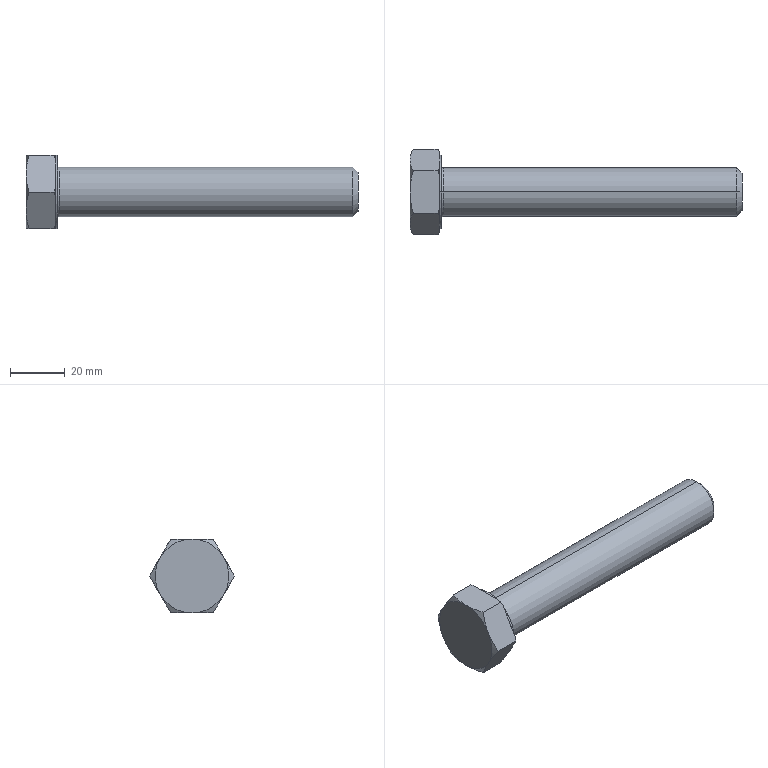Part | SolidWorks | features RevCut 4, Chamfer 1, Extrusion 1, Fillet 1, LPattern 1, Revolution 1 | 1 solid | 35 faces | box 121.5 x 31.177 x 27 mm | volume 35083 mm3 | plane 15 | cone 14 | cylinder 4 | torus 2 | commonest cylinder face diameters 18 x2 27 x2
STEP:
#1=CARTESIAN_POINT('',(12.1,0.,9.));
#2=VERTEX_POINT('',#1);
#3=CARTESIAN_POINT('',(12.1,0.,-9.));
#4=VERTEX_POINT('',#3);
#5=CARTESIAN_POINT('',(12.1,0.,0.));
#6=DIRECTION('',(1.,0.,0.));
#7=DIRECTION('',(0.,0.,-1.));
#8=AXIS2_PLACEMENT_3D('',#5,#6,#7);
#9=CIRCLE('',#8,9.);
#10=EDGE_CURVE('',#2,#4,#9,.T.);
#11=ORIENTED_EDGE('',*,*,#10,.F.);
#12=CARTESIAN_POINT('',(11.5,0.,9.6));
#13=VERTEX_POINT('',#12);
#14=CARTESIAN_POINT('',(12.1,0.,9.6));
#15=DIRECTION('',(0.,1.,0.));
#16=DIRECTION('',(0.,0.,1.));
#17=AXIS2_PLACEMENT_3D('',#14,#15,#16);
#18=CIRCLE('',#17,0.6);
#19=EDGE_CURVE('',#2,#13,#18,.T.);
#20=ORIENTED_EDGE('',*,*,#19,.T.);
#21=CARTESIAN_POINT('',(11.5,0.,-9.6));
#22=VERTEX_POINT('',#21);
#23=CARTESIAN_POINT('',(11.5,0.,0.));
#24=DIRECTION('',(-1.,0.,0.));
#25=DIRECTION('',(0.,0.,-1.));
#26=AXIS2_PLACEMENT_3D('',#23,#24,#25);
#27=CIRCLE('',#26,9.6);
#28=EDGE_CURVE('',#22,#13,#27,.T.);
#29=ORIENTED_EDGE('',*,*,#28,.F.);
#30=CARTESIAN_POINT('',(12.1,0.,-9.6));
#31=DIRECTION('',(0.,-1.,0.));
#32=DIRECTION('',(0.,0.,-1.));
#33=AXIS2_PLACEMENT_3D('',#30,#31,#32);
#34=CIRCLE('',#33,0.6);
#35=EDGE_CURVE('',#4,#22,#34,.T.);
#36=ORIENTED_EDGE('',*,*,#35,.F.);
#37=EDGE_LOOP('',(#11,#20,#29,#36));
#38=FACE_OUTER_BOUND('',#37,.T.);
#39=CARTESIAN_POINT('',(12.1,0.,0.));
#40=DIRECTION('',(1.,0.,0.));
#41=DIRECTION('',(0.,0.,-1.));
#42=AXIS2_PLACEMENT_3D('',#39,#40,#41);
#43=TOROIDAL_SURFACE('',#42,9.6,0.6);
#44=ADVANCED_FACE('',(#38),#43,.F.);
#45=CARTESIAN_POINT('',(121.5,0.,-7.));
#46=VERTEX_POINT('',#45);
#47=CARTESIAN_POINT('',(121.5,0.,7.));
#48=VERTEX_POINT('',#47);
#49=CARTESIAN_POINT('',(121.5,0.,0.));
#50=DIRECTION('',(1.,0.,0.));
#51=DIRECTION('',(0.,0.,1.));
#52=AXIS2_PLACEMENT_3D('',#49,#50,#51);
#53=CIRCLE('',#52,7.);
#54=EDGE_CURVE('',#46,#48,#53,.T.);
#55=ORIENTED_EDGE('',*,*,#54,.F.);
#56=CARTESIAN_POINT('',(119.5,0.,-9.));
#57=VERTEX_POINT('',#56);
#58=CARTESIAN_POINT('',(119.5,0.,-9.));
#59=DIRECTION('',(-0.7071,0.,-0.7071));
#60=VECTOR('',#59,1000.);
#61=LINE('',#58,#60);
#62=EDGE_CURVE('',#46,#57,#61,.T.);
#63=ORIENTED_EDGE('',*,*,#62,.T.);
#64=CARTESIAN_POINT('',(119.5,0.,9.));
#65=VERTEX_POINT('',#64);
#66=CARTESIAN_POINT('',(119.5,0.,0.));
#67=DIRECTION('',(-1.,0.,0.));
#68=DIRECTION('',(0.,0.,1.));
#69=AXIS2_PLACEMENT_3D('',#66,#67,#68);
#70=CIRCLE('',#69,9.);
#71=EDGE_CURVE('',#65,#57,#70,.T.);
#72=ORIENTED_EDGE('',*,*,#71,.F.);
#73=CARTESIAN_POINT('',(119.5,0.,9.));
#74=DIRECTION('',(-0.7071,0.,0.7071));
#75=VECTOR('',#74,1000.);
#76=LINE('',#73,#75);
#77=EDGE_CURVE('',#48,#65,#76,.T.);
#78=ORIENTED_EDGE('',*,*,#77,.F.);
#79=EDGE_LOOP('',(#55,#63,#72,#78));
#80=FACE_OUTER_BOUND('',#79,.T.);
#81=CARTESIAN_POINT('',(119.5,0.,0.));
#82=DIRECTION('',(-1.,0.,0.));
#83=DIRECTION('',(0.,0.,1.));
#84=AXIS2_PLACEMENT_3D('',#81,#82,#83);
#85=CONICAL_SURFACE('',#84,9.,0.7854);
#86=ADVANCED_FACE('',(#80),#85,.T.);
#87=ORIENTED_EDGE('',*,*,#71,.T.);
#88=CARTESIAN_POINT('',(0.,0.,-9.));
#89=DIRECTION('',(-1.,0.,0.));
#90=VECTOR('',#89,1000.);
#91=LINE('',#88,#90);
#92=EDGE_CURVE('',#57,#4,#91,.T.);
#93=ORIENTED_EDGE('',*,*,#92,.T.);
#94=CARTESIAN_POINT('',(12.1,0.,0.));
#95=DIRECTION('',(1.,0.,0.));
#96=DIRECTION('',(0.,0.,-1.));
#97=AXIS2_PLACEMENT_3D('',#94,#95,#96);
#98=CIRCLE('',#97,9.);
#99=EDGE_CURVE('',#4,#2,#98,.T.);
#100=ORIENTED_EDGE('',*,*,#99,.T.);
#101=CARTESIAN_POINT('',(0.,0.,9.));
#102=DIRECTION('',(-1.,0.,0.));
#103=VECTOR('',#102,1000.);
#104=LINE('',#101,#103);
#105=EDGE_CURVE('',#65,#2,#104,.T.);
#106=ORIENTED_EDGE('',*,*,#105,.F.);
#107=EDGE_LOOP('',(#87,#93,#100,#106));
#108=FACE_OUTER_BOUND('',#107,.T.);
#109=CARTESIAN_POINT('',(0.,0.,0.));
#110=DIRECTION('',(-1.,0.,0.));
#111=DIRECTION('',(0.,0.,1.));
#112=AXIS2_PLACEMENT_3D('',#109,#110,#111);
#113=CYLINDRICAL_SURFACE('',#112,9.);
#114=ADVANCED_FACE('',(#108),#113,.T.);
#115=CARTESIAN_POINT('',(11.5,0.,-13.5));
#116=VERTEX_POINT('',#115);
#117=CARTESIAN_POINT('',(11.5,0.,13.5));
#118=VERTEX_POINT('',#117);
#119=CARTESIAN_POINT('',(11.5,0.,0.));
#120=DIRECTION('',(1.,0.,0.));
#121=DIRECTION('',(0.,0.,-1.));
#122=AXIS2_PLACEMENT_3D('',#119,#120,#121);
#123=CIRCLE('',#122,13.5);
#124=EDGE_CURVE('',#116,#118,#123,.T.);
#125=ORIENTED_EDGE('',*,*,#124,.F.);
#126=CARTESIAN_POINT('',(10.7,0.,-13.5));
#127=VERTEX_POINT('',#126);
#128=CARTESIAN_POINT('',(0.,0.,-13.5));
#129=DIRECTION('',(-1.,0.,0.));
#130=VECTOR('',#129,1000.);
#131=LINE('',#128,#130);
#132=EDGE_CURVE('',#116,#127,#131,.T.);
#133=ORIENTED_EDGE('',*,*,#132,.T.);
#134=CARTESIAN_POINT('',(10.7,11.691,-6.75));
#135=VERTEX_POINT('',#134);
#136=CARTESIAN_POINT('',(10.7,0.,0.));
#137=DIRECTION('',(-1.,0.,0.));
#138=DIRECTION('',(0.,0.,1.));
#139=AXIS2_PLACEMENT_3D('',#136,#137,#138);
#140=CIRCLE('',#139,13.5);
#141=EDGE_CURVE('',#135,#127,#140,.T.);
#142=ORIENTED_EDGE('',*,*,#141,.F.);
#143=CARTESIAN_POINT('',(10.7,11.691,6.75));
#144=VERTEX_POINT('',#143);
#145=CARTESIAN_POINT('',(10.7,0.,0.));
#146=DIRECTION('',(-1.,0.,0.));
#147=DIRECTION('',(0.,0.,1.));
#148=AXIS2_PLACEMENT_3D('',#145,#146,#147);
#149=CIRCLE('',#148,13.5);
#150=EDGE_CURVE('',#144,#135,#149,.T.);
#151=ORIENTED_EDGE('',*,*,#150,.F.);
#152=CARTESIAN_POINT('',(10.7,0.,13.5));
#153=VERTEX_POINT('',#152);
#154=CARTESIAN_POINT('',(10.7,0.,0.));
#155=DIRECTION('',(-1.,0.,0.));
#156=DIRECTION('',(0.,0.,1.));
#157=AXIS2_PLACEMENT_3D('',#154,#155,#156);
#158=CIRCLE('',#157,13.5);
#159=EDGE_CURVE('',#153,#144,#158,.T.);
#160=ORIENTED_EDGE('',*,*,#159,.F.);
#161=CARTESIAN_POINT('',(0.,0.,13.5));
#162=DIRECTION('',(-1.,0.,0.));
#163=VECTOR('',#162,1000.);
#164=LINE('',#161,#163);
#165=EDGE_CURVE('',#118,#153,#164,.T.);
#166=ORIENTED_EDGE('',*,*,#165,.F.);
#167=EDGE_LOOP('',(#125,#133,#142,#151,#160,#166));
#168=FACE_OUTER_BOUND('',#167,.T.);
#169=CARTESIAN_POINT('',(0.,0.,0.));
#170=DIRECTION('',(-1.,0.,0.));
#171=DIRECTION('',(0.,0.,1.));
#172=AXIS2_PLACEMENT_3D('',#169,#170,#171);
#173=CYLINDRICAL_SURFACE('',#172,13.5);
#174=ADVANCED_FACE('',(#168),#173,.T.);
#175=CARTESIAN_POINT('',(10.7,8.556,-12.181));
#176=VERTEX_POINT('',#175);
#177=CARTESIAN_POINT('',(10.7,7.794,-13.5));
#178=DIRECTION('',(0.,0.5,0.866));
#179=VECTOR('',#178,1000.);
#180=LINE('',#177,#179);
#181=EDGE_CURVE('',#176,#135,#180,.T.);
#182=ORIENTED_EDGE('',*,*,#181,.F.);
#183=CARTESIAN_POINT('',(10.294,7.794,-13.5));
#184=VERTEX_POINT('',#183);
#185=CARTESIAN_POINT('',(10.294,7.794,-13.5));
#186=CARTESIAN_POINT('',(10.44,8.047,-13.062));
#187=CARTESIAN_POINT('',(10.576,8.301,-12.622));
#188=CARTESIAN_POINT('',(10.7,8.556,-12.181));
#189=B_SPLINE_CURVE_WITH_KNOTS('',3,(#185,#186,#187,#188),.UNSPECIFIED.,.F.,.F.,(4,4),(0.000000238,0.001565),.UNSPECIFIED.);
#190=EDGE_CURVE('',#184,#176,#189,.T.);
#191=ORIENTED_EDGE('',*,*,#190,.F.);
#192=CARTESIAN_POINT('',(1.206,7.794,-13.5));
#193=VERTEX_POINT('',#192);
#194=CARTESIAN_POINT('',(11.5,7.794,-13.5));
#195=DIRECTION('',(-1.,0.,0.));
#196=VECTOR('',#195,1000.);
#197=LINE('',#194,#196);
#198=EDGE_CURVE('',#184,#193,#197,.T.);
#199=ORIENTED_EDGE('',*,*,#198,.T.);
#200=CARTESIAN_POINT('',(0.,11.691,-6.75));
#201=VERTEX_POINT('',#200);
#202=CARTESIAN_POINT('',(0.,11.691,-6.75));
#203=CARTESIAN_POINT('',(0.,11.361,-7.323));
#204=CARTESIAN_POINT('',(0.0285,11.028,-7.898));
#205=CARTESIAN_POINT('',(0.1388,10.371,-9.037));
#206=CARTESIAN_POINT('',(0.2205,10.045,-9.602));
#207=CARTESIAN_POINT('',(0.5355,9.071,-11.288));
#208=CARTESIAN_POINT('',(0.8386,8.43,-12.399));
#209=CARTESIAN_POINT('',(1.206,7.794,-13.5));
#210=B_SPLINE_CURVE_WITH_KNOTS('',3,(#202,#203,#204,#205,#206,#207,#208,#209),.UNSPECIFIED.,.F.,.F.,(4,2,2,4),(0.007887,0.009851,0.01182,0.01574),.UNSPECIFIED.);
#211=EDGE_CURVE('',#201,#193,#210,.T.);
#212=ORIENTED_EDGE('',*,*,#211,.F.);
#213=CARTESIAN_POINT('',(1.206,15.588,0.));
#214=VERTEX_POINT('',#213);
#215=CARTESIAN_POINT('',(1.206,15.588,0.));
#216=CARTESIAN_POINT('',(0.8377,14.951,-1.104));
#217=CARTESIAN_POINT('',(0.5345,14.309,-2.216));
#218=CARTESIAN_POINT('',(0.1149,13.011,-4.464));
#219=CARTESIAN_POINT('',(0.,12.355,-5.6));
#220=CARTESIAN_POINT('',(0.,11.691,-6.75));
#221=B_SPLINE_CURVE_WITH_KNOTS('',3,(#215,#216,#217,#218,#219,#220),.UNSPECIFIED.,.F.,.F.,(4,2,4),(0.000000238,0.003943,0.007887),.UNSPECIFIED.);
#222=EDGE_CURVE('',#214,#201,#221,.T.);
#223=ORIENTED_EDGE('',*,*,#222,.F.);
#224=CARTESIAN_POINT('',(10.294,15.588,0.));
#225=VERTEX_POINT('',#224);
#226=CARTESIAN_POINT('',(11.5,15.588,0.));
#227=DIRECTION('',(-1.,0.,0.));
#228=VECTOR('',#227,1000.);
#229=LINE('',#226,#228);
#230=EDGE_CURVE('',#225,#214,#229,.T.);
#231=ORIENTED_EDGE('',*,*,#230,.F.);
#232=CARTESIAN_POINT('',(10.7,14.827,-1.319));
#233=VERTEX_POINT('',#232);
#234=CARTESIAN_POINT('',(10.7,14.827,-1.319));
#235=CARTESIAN_POINT('',(10.576,15.082,-0.8775));
#236=CARTESIAN_POINT('',(10.44,15.336,-0.438));
#237=CARTESIAN_POINT('',(10.294,15.588,0.));
#238=B_SPLINE_CURVE_WITH_KNOTS('',3,(#234,#235,#236,#237),.UNSPECIFIED.,.F.,.F.,(4,4),(0.01418,0.01574),.UNSPECIFIED.);
#239=EDGE_CURVE('',#233,#225,#238,.T.);
#240=ORIENTED_EDGE('',*,*,#239,.F.);
#241=CARTESIAN_POINT('',(10.7,7.794,-13.5));
#242=DIRECTION('',(0.,0.5,0.866));
#243=VECTOR('',#242,1000.);
#244=LINE('',#241,#243);
#245=EDGE_CURVE('',#135,#233,#244,.T.);
#246=ORIENTED_EDGE('',*,*,#245,.F.);
#247=EDGE_LOOP('',(#182,#191,#199,#212,#223,#231,#240,#246));
#248=FACE_OUTER_BOUND('',#247,.T.);
#249=CARTESIAN_POINT('',(11.5,7.794,-13.5));
#250=DIRECTION('',(0.,-0.866,0.5));
#251=DIRECTION('',(0.,-0.5,-0.866));
#252=AXIS2_PLACEMENT_3D('',#249,#250,#251);
#253=PLANE('',#252);
#254=ADVANCED_FACE('',(#248),#253,.F.);
#255=CARTESIAN_POINT('',(10.7,14.827,1.319));
#256=VERTEX_POINT('',#255);
#257=CARTESIAN_POINT('',(10.7,15.588,0.));
#258=DIRECTION('',(0.,-0.5,0.866));
#259=VECTOR('',#258,1000.);
#260=LINE('',#257,#259);
#261=EDGE_CURVE('',#256,#144,#260,.T.);
#262=ORIENTED_EDGE('',*,*,#261,.F.);
#263=CARTESIAN_POINT('',(10.294,15.588,0.));
#264=CARTESIAN_POINT('',(10.44,15.335,0.4382));
#265=CARTESIAN_POINT('',(10.576,15.082,0.8777));
#266=CARTESIAN_POINT('',(10.7,14.827,1.319));
#267=B_SPLINE_CURVE_WITH_KNOTS('',3,(#263,#264,#265,#266),.UNSPECIFIED.,.F.,.F.,(4,4),(0.000000238,0.001565),.UNSPECIFIED.);
#268=EDGE_CURVE('',#225,#256,#267,.T.);
#269=ORIENTED_EDGE('',*,*,#268,.F.);
#270=ORIENTED_EDGE('',*,*,#230,.T.);
#271=CARTESIAN_POINT('',(0.,11.691,6.75));
#272=VERTEX_POINT('',#271);
#273=CARTESIAN_POINT('',(0.,11.691,6.75));
#274=CARTESIAN_POINT('',(0.,12.022,6.177));
#275=CARTESIAN_POINT('',(0.0285,12.354,5.602));
#276=CARTESIAN_POINT('',(0.1388,13.011,4.463));
#277=CARTESIAN_POINT('',(0.2205,13.338,3.898));
#278=CARTESIAN_POINT('',(0.5355,14.311,2.212));
#279=CARTESIAN_POINT('',(0.8386,14.953,1.101));
#280=CARTESIAN_POINT('',(1.206,15.588,0.));
#281=B_SPLINE_CURVE_WITH_KNOTS('',3,(#273,#274,#275,#276,#277,#278,#279,#280),.UNSPECIFIED.,.F.,.F.,(4,2,2,4),(0.007887,0.009851,0.01182,0.01574),.UNSPECIFIED.);
#282=EDGE_CURVE('',#272,#214,#281,.T.);
#283=ORIENTED_EDGE('',*,*,#282,.F.);
#284=CARTESIAN_POINT('',(1.206,7.794,13.5));
#285=VERTEX_POINT('',#284);
#286=CARTESIAN_POINT('',(1.206,7.794,13.5));
#287=CARTESIAN_POINT('',(0.8377,8.432,12.396));
#288=CARTESIAN_POINT('',(0.5345,9.074,11.284));
#289=CARTESIAN_POINT('',(0.1149,10.372,9.036));
#290=CARTESIAN_POINT('',(0.,11.027,7.9));
#291=CARTESIAN_POINT('',(0.,11.691,6.75));
#292=B_SPLINE_CURVE_WITH_KNOTS('',3,(#286,#287,#288,#289,#290,#291),.UNSPECIFIED.,.F.,.F.,(4,2,4),(0.000000238,0.003943,0.007887),.UNSPECIFIED.);
#293=EDGE_CURVE('',#285,#272,#292,.T.);
#294=ORIENTED_EDGE('',*,*,#293,.F.);
#295=CARTESIAN_POINT('',(10.294,7.794,13.5));
#296=VERTEX_POINT('',#295);
#297=CARTESIAN_POINT('',(11.5,7.794,13.5));
#298=DIRECTION('',(-1.,0.,0.));
#299=VECTOR('',#298,1000.);
#300=LINE('',#297,#299);
#301=EDGE_CURVE('',#296,#285,#300,.T.);
#302=ORIENTED_EDGE('',*,*,#301,.F.);
#303=CARTESIAN_POINT('',(10.7,8.556,12.181));
#304=VERTEX_POINT('',#303);
#305=CARTESIAN_POINT('',(10.7,8.556,12.181));
#306=CARTESIAN_POINT('',(10.576,8.301,12.623));
#307=CARTESIAN_POINT('',(10.44,8.047,13.062));
#308=CARTESIAN_POINT('',(10.294,7.794,13.5));
#309=B_SPLINE_CURVE_WITH_KNOTS('',3,(#305,#306,#307,#308),.UNSPECIFIED.,.F.,.F.,(4,4),(0.01418,0.01574),.UNSPECIFIED.);
#310=EDGE_CURVE('',#304,#296,#309,.T.);
#311=ORIENTED_EDGE('',*,*,#310,.F.);
#312=CARTESIAN_POINT('',(10.7,15.588,0.));
#313=DIRECTION('',(0.,-0.5,0.866));
#314=VECTOR('',#313,1000.);
#315=LINE('',#312,#314);
#316=EDGE_CURVE('',#144,#304,#315,.T.);
#317=ORIENTED_EDGE('',*,*,#316,.F.);
#318=EDGE_LOOP('',(#262,#269,#270,#283,#294,#302,#311,#317));
#319=FACE_OUTER_BOUND('',#318,.T.);
#320=CARTESIAN_POINT('',(11.5,15.588,0.));
#321=DIRECTION('',(0.,-0.866,-0.5));
#322=DIRECTION('',(0.,0.5,-0.866));
#323=AXIS2_PLACEMENT_3D('',#320,#321,#322);
#324=PLANE('',#323);
#325=ADVANCED_FACE('',(#319),#324,.F.);
#326=CARTESIAN_POINT('',(10.7,6.272,13.5));
#327=VERTEX_POINT('',#326);
#328=CARTESIAN_POINT('',(10.7,7.794,13.5));
#329=DIRECTION('',(0.,-1.,0.));
#330=VECTOR('',#329,1000.);
#331=LINE('',#328,#330);
#332=EDGE_CURVE('',#327,#153,#331,.T.);
#333=ORIENTED_EDGE('',*,*,#332,.F.);
#334=CARTESIAN_POINT('',(10.294,7.794,13.5));
#335=CARTESIAN_POINT('',(10.44,7.289,13.5));
#336=CARTESIAN_POINT('',(10.576,6.782,13.5));
#337=CARTESIAN_POINT('',(10.7,6.272,13.5));
#338=B_SPLINE_CURVE_WITH_KNOTS('',3,(#334,#335,#336,#337),.UNSPECIFIED.,.F.,.F.,(4,4),(0.03601,0.03759),.UNSPECIFIED.);
#339=EDGE_CURVE('',#296,#327,#338,.T.);
#340=ORIENTED_EDGE('',*,*,#339,.F.);
#341=ORIENTED_EDGE('',*,*,#301,.T.);
#342=CARTESIAN_POINT('',(0.,0.,13.5));
#343=VERTEX_POINT('',#342);
#344=CARTESIAN_POINT('',(0.,0.,13.5));
#345=CARTESIAN_POINT('',(0.,0.6597,13.5));
#346=CARTESIAN_POINT('',(0.02816,1.323,13.5));
#347=CARTESIAN_POINT('',(0.1397,2.65,13.5));
#348=CARTESIAN_POINT('',(0.2222,3.306,13.5));
#349=CARTESIAN_POINT('',(0.539,5.257,13.5));
#350=CARTESIAN_POINT('',(0.8419,6.534,13.5));
#351=CARTESIAN_POINT('',(1.206,7.794,13.5));
#352=B_SPLINE_CURVE_WITH_KNOTS('',3,(#344,#345,#346,#347,#348,#349,#350,#351),.UNSPECIFIED.,.F.,.F.,(4,2,2,4),(0.02224,0.02422,0.02619,0.03014),.UNSPECIFIED.);
#353=EDGE_CURVE('',#343,#285,#352,.T.);
#354=ORIENTED_EDGE('',*,*,#353,.F.);
#355=CARTESIAN_POINT('',(1.206,-7.794,13.5));
#356=VERTEX_POINT('',#355);
#357=CARTESIAN_POINT('',(1.206,-7.794,13.5));
#358=CARTESIAN_POINT('',(0.8395,-6.525,13.5));
#359=CARTESIAN_POINT('',(0.5328,-5.228,13.5));
#360=CARTESIAN_POINT('',(0.1134,-2.627,13.5));
#361=CARTESIAN_POINT('',(0.,-1.318,13.5));
#362=CARTESIAN_POINT('',(0.,0.,13.5));
#363=B_SPLINE_CURVE_WITH_KNOTS('',3,(#357,#358,#359,#360,#361,#362),.UNSPECIFIED.,.F.,.F.,(4,2,4),(0.01435,0.0183,0.02224),.UNSPECIFIED.);
#364=EDGE_CURVE('',#356,#343,#363,.T.);
#365=ORIENTED_EDGE('',*,*,#364,.F.);
#366=CARTESIAN_POINT('',(10.294,-7.794,13.5));
#367=VERTEX_POINT('',#366);
#368=CARTESIAN_POINT('',(11.5,-7.794,13.5));
#369=DIRECTION('',(-1.,0.,0.));
#370=VECTOR('',#369,1000.);
#371=LINE('',#368,#370);
#372=EDGE_CURVE('',#367,#356,#371,.T.);
#373=ORIENTED_EDGE('',*,*,#372,.F.);
#374=CARTESIAN_POINT('',(10.7,-6.272,13.5));
#375=VERTEX_POINT('',#374);
#376=CARTESIAN_POINT('',(10.7,-6.272,13.5));
#377=CARTESIAN_POINT('',(10.576,-6.783,13.5));
#378=CARTESIAN_POINT('',(10.44,-7.291,13.5));
#379=CARTESIAN_POINT('',(10.294,-7.794,13.5));
#380=B_SPLINE_CURVE_WITH_KNOTS('',3,(#376,#377,#378,#379),.UNSPECIFIED.,.F.,.F.,(4,4),(0.05024,0.0518),.UNSPECIFIED.);
#381=EDGE_CURVE('',#375,#367,#380,.T.);
#382=ORIENTED_EDGE('',*,*,#381,.F.);
#383=CARTESIAN_POINT('',(10.7,7.794,13.5));
#384=DIRECTION('',(0.,-1.,0.));
#385=VECTOR('',#384,1000.);
#386=LINE('',#383,#385);
#387=EDGE_CURVE('',#153,#375,#386,.T.);
#388=ORIENTED_EDGE('',*,*,#387,.F.);
#389=EDGE_LOOP('',(#333,#340,#341,#354,#365,#373,#382,#388));
#390=FACE_OUTER_BOUND('',#389,.T.);
#391=CARTESIAN_POINT('',(11.5,7.794,13.5));
#392=DIRECTION('',(0.,0.,-1.));
#393=DIRECTION('',(-1.,0.,0.));
#394=AXIS2_PLACEMENT_3D('',#391,#392,#393);
#395=PLANE('',#394);
#396=ADVANCED_FACE('',(#390),#395,.F.);
#397=CARTESIAN_POINT('',(10.7,-8.556,12.181));
#398=VERTEX_POINT('',#397);
#399=CARTESIAN_POINT('',(10.7,-11.691,6.75));
#400=VERTEX_POINT('',#399);
#401=CARTESIAN_POINT('',(10.7,-15.588,0.));
#402=DIRECTION('',(0.,-0.5,-0.866));
#403=VECTOR('',#402,1000.);
#404=LINE('',#401,#403);
#405=EDGE_CURVE('',#398,#400,#404,.T.);
#406=ORIENTED_EDGE('',*,*,#405,.F.);
#407=CARTESIAN_POINT('',(10.294,-7.794,13.5));
#408=CARTESIAN_POINT('',(10.44,-8.047,13.062));
#409=CARTESIAN_POINT('',(10.576,-8.301,12.622));
#410=CARTESIAN_POINT('',(10.7,-8.556,12.181));
#411=B_SPLINE_CURVE_WITH_KNOTS('',3,(#407,#408,#409,#410),.UNSPECIFIED.,.F.,.F.,(4,4),(0.000000238,0.001565),.UNSPECIFIED.);
#412=EDGE_CURVE('',#367,#398,#411,.T.);
#413=ORIENTED_EDGE('',*,*,#412,.F.);
#414=ORIENTED_EDGE('',*,*,#372,.T.);
#415=CARTESIAN_POINT('',(0.,-11.691,6.75));
#416=VERTEX_POINT('',#415);
#417=CARTESIAN_POINT('',(0.,-11.691,6.75));
#418=CARTESIAN_POINT('',(0.,-11.361,7.323));
#419=CARTESIAN_POINT('',(0.0285,-11.028,7.898));
#420=CARTESIAN_POINT('',(0.1388,-10.371,9.037));
#421=CARTESIAN_POINT('',(0.2205,-10.045,9.602));
#422=CARTESIAN_POINT('',(0.5355,-9.071,11.288));
#423=CARTESIAN_POINT('',(0.8386,-8.43,12.399));
#424=CARTESIAN_POINT('',(1.206,-7.794,13.5));
#425=B_SPLINE_CURVE_WITH_KNOTS('',3,(#417,#418,#419,#420,#421,#422,#423,#424),.UNSPECIFIED.,.F.,.F.,(4,2,2,4),(0.007887,0.009851,0.01182,0.01574),.UNSPECIFIED.);
#426=EDGE_CURVE('',#416,#356,#425,.T.);
#427=ORIENTED_EDGE('',*,*,#426,.F.);
#428=CARTESIAN_POINT('',(1.206,-15.588,0.));
#429=VERTEX_POINT('',#428);
#430=CARTESIAN_POINT('',(1.206,-15.588,0.));
#431=CARTESIAN_POINT('',(0.8377,-14.951,1.104));
#432=CARTESIAN_POINT('',(0.5345,-14.309,2.216));
#433=CARTESIAN_POINT('',(0.1149,-13.011,4.464));
#434=CARTESIAN_POINT('',(0.,-12.355,5.6));
#435=CARTESIAN_POINT('',(0.,-11.691,6.75));
#436=B_SPLINE_CURVE_WITH_KNOTS('',3,(#430,#431,#432,#433,#434,#435),.UNSPECIFIED.,.F.,.F.,(4,2,4),(0.000000238,0.003943,0.007887),.UNSPECIFIED.);
#437=EDGE_CURVE('',#429,#416,#436,.T.);
#438=ORIENTED_EDGE('',*,*,#437,.F.);
#439=CARTESIAN_POINT('',(10.294,-15.588,0.));
#440=VERTEX_POINT('',#439);
#441=CARTESIAN_POINT('',(11.5,-15.588,0.));
#442=DIRECTION('',(-1.,0.,0.));
#443=VECTOR('',#442,1000.);
#444=LINE('',#441,#443);
#445=EDGE_CURVE('',#440,#429,#444,.T.);
#446=ORIENTED_EDGE('',*,*,#445,.F.);
#447=CARTESIAN_POINT('',(10.7,-14.827,1.319));
#448=VERTEX_POINT('',#447);
#449=CARTESIAN_POINT('',(10.7,-14.827,1.319));
#450=CARTESIAN_POINT('',(10.576,-15.082,0.8775));
#451=CARTESIAN_POINT('',(10.44,-15.336,0.438));
#452=CARTESIAN_POINT('',(10.294,-15.588,0.));
#453=B_SPLINE_CURVE_WITH_KNOTS('',3,(#449,#450,#451,#452),.UNSPECIFIED.,.F.,.F.,(4,4),(0.01418,0.01574),.UNSPECIFIED.);
#454=EDGE_CURVE('',#448,#440,#453,.T.);
#455=ORIENTED_EDGE('',*,*,#454,.F.);
#456=CARTESIAN_POINT('',(10.7,-15.588,0.));
#457=DIRECTION('',(0.,-0.5,-0.866));
#458=VECTOR('',#457,1000.);
#459=LINE('',#456,#458);
#460=EDGE_CURVE('',#400,#448,#459,.T.);
#461=ORIENTED_EDGE('',*,*,#460,.F.);
#462=EDGE_LOOP('',(#406,#413,#414,#427,#438,#446,#455,#461));
#463=FACE_OUTER_BOUND('',#462,.T.);
#464=CARTESIAN_POINT('',(11.5,-15.588,0.));
#465=DIRECTION('',(0.,0.866,-0.5));
#466=DIRECTION('',(0.,0.5,0.866));
#467=AXIS2_PLACEMENT_3D('',#464,#465,#466);
#468=PLANE('',#467);
#469=ADVANCED_FACE('',(#463),#468,.F.);
#470=CARTESIAN_POINT('',(10.7,-14.827,-1.319));
#471=VERTEX_POINT('',#470);
#472=CARTESIAN_POINT('',(10.7,-11.691,-6.75));
#473=VERTEX_POINT('',#472);
#474=CARTESIAN_POINT('',(10.7,-7.794,-13.5));
#475=DIRECTION('',(0.,0.5,-0.866));
#476=VECTOR('',#475,1000.);
#477=LINE('',#474,#476);
#478=EDGE_CURVE('',#471,#473,#477,.T.);
#479=ORIENTED_EDGE('',*,*,#478,.F.);
#480=CARTESIAN_POINT('',(10.294,-15.588,0.));
#481=CARTESIAN_POINT('',(10.44,-15.335,-0.4382));
#482=CARTESIAN_POINT('',(10.576,-15.082,-0.8777));
#483=CARTESIAN_POINT('',(10.7,-14.827,-1.319));
#484=B_SPLINE_CURVE_WITH_KNOTS('',3,(#480,#481,#482,#483),.UNSPECIFIED.,.F.,.F.,(4,4),(0.000000238,0.001565),.UNSPECIFIED.);
#485=EDGE_CURVE('',#440,#471,#484,.T.);
#486=ORIENTED_EDGE('',*,*,#485,.F.);
#487=ORIENTED_EDGE('',*,*,#445,.T.);
#488=CARTESIAN_POINT('',(0.,-11.691,-6.75));
#489=VERTEX_POINT('',#488);
#490=CARTESIAN_POINT('',(0.,-11.691,-6.75));
#491=CARTESIAN_POINT('',(0.,-12.022,-6.177));
#492=CARTESIAN_POINT('',(0.0285,-12.354,-5.602));
#493=CARTESIAN_POINT('',(0.1388,-13.011,-4.463));
#494=CARTESIAN_POINT('',(0.2205,-13.338,-3.898));
#495=CARTESIAN_POINT('',(0.5355,-14.311,-2.212));
#496=CARTESIAN_POINT('',(0.8386,-14.953,-1.101));
#497=CARTESIAN_POINT('',(1.206,-15.588,0.));
#498=B_SPLINE_CURVE_WITH_KNOTS('',3,(#490,#491,#492,#493,#494,#495,#496,#497),.UNSPECIFIED.,.F.,.F.,(4,2,2,4),(0.007887,0.009851,0.01182,0.01574),.UNSPECIFIED.);
#499=EDGE_CURVE('',#489,#429,#498,.T.);
#500=ORIENTED_EDGE('',*,*,#499,.F.);
#501=CARTESIAN_POINT('',(1.206,-7.794,-13.5));
#502=VERTEX_POINT('',#501);
#503=CARTESIAN_POINT('',(1.206,-7.794,-13.5));
#504=CARTESIAN_POINT('',(0.8377,-8.432,-12.396));
#505=CARTESIAN_POINT('',(0.5345,-9.074,-11.284));
#506=CARTESIAN_POINT('',(0.1149,-10.372,-9.036));
#507=CARTESIAN_POINT('',(0.,-11.027,-7.9));
#508=CARTESIAN_POINT('',(0.,-11.691,-6.75));
#509=B_SPLINE_CURVE_WITH_KNOTS('',3,(#503,#504,#505,#506,#507,#508),.UNSPECIFIED.,.F.,.F.,(4,2,4),(0.000000238,0.003943,0.007887),.UNSPECIFIED.);
#510=EDGE_CURVE('',#502,#489,#509,.T.);
#511=ORIENTED_EDGE('',*,*,#510,.F.);
#512=CARTESIAN_POINT('',(10.294,-7.794,-13.5));
#513=VERTEX_POINT('',#512);
#514=CARTESIAN_POINT('',(11.5,-7.794,-13.5));
#515=DIRECTION('',(-1.,0.,0.));
#516=VECTOR('',#515,1000.);
#517=LINE('',#514,#516);
#518=EDGE_CURVE('',#513,#502,#517,.T.);
#519=ORIENTED_EDGE('',*,*,#518,.F.);
#520=CARTESIAN_POINT('',(10.7,-8.556,-12.181));
#521=VERTEX_POINT('',#520);
#522=CARTESIAN_POINT('',(10.7,-8.556,-12.181));
#523=CARTESIAN_POINT('',(10.576,-8.301,-12.623));
#524=CARTESIAN_POINT('',(10.44,-8.047,-13.062));
#525=CARTESIAN_POINT('',(10.294,-7.794,-13.5));
#526=B_SPLINE_CURVE_WITH_KNOTS('',3,(#522,#523,#524,#525),.UNSPECIFIED.,.F.,.F.,(4,4),(0.01418,0.01574),.UNSPECIFIED.);
#527=EDGE_CURVE('',#521,#513,#526,.T.);
#528=ORIENTED_EDGE('',*,*,#527,.F.);
#529=CARTESIAN_POINT('',(10.7,-7.794,-13.5));
#530=DIRECTION('',(0.,0.5,-0.866));
#531=VECTOR('',#530,1000.);
#532=LINE('',#529,#531);
#533=EDGE_CURVE('',#473,#521,#532,.T.);
#534=ORIENTED_EDGE('',*,*,#533,.F.);
#535=EDGE_LOOP('',(#479,#486,#487,#500,#511,#519,#528,#534));
#536=FACE_OUTER_BOUND('',#535,.T.);
#537=CARTESIAN_POINT('',(11.5,-7.794,-13.5));
#538=DIRECTION('',(0.,0.866,0.5));
#539=DIRECTION('',(0.,-0.5,0.866));
#540=AXIS2_PLACEMENT_3D('',#537,#538,#539);
#541=PLANE('',#540);
#542=ADVANCED_FACE('',(#536),#541,.F.);
#543=CARTESIAN_POINT('',(10.7,-6.272,-13.5));
#544=VERTEX_POINT('',#543);
#545=CARTESIAN_POINT('',(10.7,7.794,-13.5));
#546=DIRECTION('',(0.,1.,0.));
#547=VECTOR('',#546,1000.);
#548=LINE('',#545,#547);
#549=EDGE_CURVE('',#544,#127,#548,.T.);
#550=ORIENTED_EDGE('',*,*,#549,.F.);
#551=CARTESIAN_POINT('',(10.294,-7.794,-13.5));
#552=CARTESIAN_POINT('',(10.44,-7.291,-13.5));
#553=CARTESIAN_POINT('',(10.576,-6.783,-13.5));
#554=CARTESIAN_POINT('',(10.7,-6.272,-13.5));
#555=B_SPLINE_CURVE_WITH_KNOTS('',3,(#551,#552,#553,#554),.UNSPECIFIED.,.F.,.F.,(4,4),(0.01435,0.01592),.UNSPECIFIED.);
#556=EDGE_CURVE('',#513,#544,#555,.T.);
#557=ORIENTED_EDGE('',*,*,#556,.F.);
#558=ORIENTED_EDGE('',*,*,#518,.T.);
#559=CARTESIAN_POINT('',(0.,0.,-13.5));
#560=VERTEX_POINT('',#559);
#561=CARTESIAN_POINT('',(0.,0.,-13.5));
#562=CARTESIAN_POINT('',(0.,-1.318,-13.5));
#563=CARTESIAN_POINT('',(0.1134,-2.627,-13.5));
#564=CARTESIAN_POINT('',(0.5328,-5.228,-13.5));
#565=CARTESIAN_POINT('',(0.8395,-6.525,-13.5));
#566=CARTESIAN_POINT('',(1.206,-7.794,-13.5));
#567=B_SPLINE_CURVE_WITH_KNOTS('',3,(#561,#562,#563,#564,#565,#566),.UNSPECIFIED.,.F.,.F.,(4,2,4),(0.04391,0.04786,0.0518),.UNSPECIFIED.);
#568=EDGE_CURVE('',#560,#502,#567,.T.);
#569=ORIENTED_EDGE('',*,*,#568,.F.);
#570=CARTESIAN_POINT('',(1.206,7.794,-13.5));
#571=CARTESIAN_POINT('',(0.8419,6.534,-13.5));
#572=CARTESIAN_POINT('',(0.539,5.257,-13.5));
#573=CARTESIAN_POINT('',(0.2222,3.306,-13.5));
#574=CARTESIAN_POINT('',(0.1397,2.65,-13.5));
#575=CARTESIAN_POINT('',(0.02816,1.323,-13.5));
#576=CARTESIAN_POINT('',(0.,0.6597,-13.5));
#577=CARTESIAN_POINT('',(0.,0.,-13.5));
#578=B_SPLINE_CURVE_WITH_KNOTS('',3,(#570,#571,#572,#573,#574,#575,#576,#577),.UNSPECIFIED.,.F.,.F.,(4,2,2,4),(0.03601,0.03996,0.04194,0.04391),.UNSPECIFIED.);
#579=EDGE_CURVE('',#193,#560,#578,.T.);
#580=ORIENTED_EDGE('',*,*,#579,.F.);
#581=ORIENTED_EDGE('',*,*,#198,.F.);
#582=CARTESIAN_POINT('',(10.7,6.272,-13.5));
#583=VERTEX_POINT('',#582);
#584=CARTESIAN_POINT('',(10.7,6.272,-13.5));
#585=CARTESIAN_POINT('',(10.576,6.782,-13.5));
#586=CARTESIAN_POINT('',(10.44,7.289,-13.5));
#587=CARTESIAN_POINT('',(10.294,7.794,-13.5));
#588=B_SPLINE_CURVE_WITH_KNOTS('',3,(#584,#585,#586,#587),.UNSPECIFIED.,.F.,.F.,(4,4),(0.02856,0.03014),.UNSPECIFIED.);
#589=EDGE_CURVE('',#583,#184,#588,.T.);
#590=ORIENTED_EDGE('',*,*,#589,.F.);
#591=CARTESIAN_POINT('',(10.7,7.794,-13.5));
#592=DIRECTION('',(0.,1.,0.));
#593=VECTOR('',#592,1000.);
#594=LINE('',#591,#593);
#595=EDGE_CURVE('',#127,#583,#594,.T.);
#596=ORIENTED_EDGE('',*,*,#595,.F.);
#597=EDGE_LOOP('',(#550,#557,#558,#569,#580,#581,#590,#596));
#598=FACE_OUTER_BOUND('',#597,.T.);
#599=CARTESIAN_POINT('',(11.5,7.794,-13.5));
#600=DIRECTION('',(0.,0.,1.));
#601=DIRECTION('',(1.,0.,0.));
#602=AXIS2_PLACEMENT_3D('',#599,#600,#601);
#603=PLANE('',#602);
#604=ADVANCED_FACE('',(#598),#603,.F.);
#605=ORIENTED_EDGE('',*,*,#556,.T.);
#606=CARTESIAN_POINT('',(10.7,0.,0.));
#607=DIRECTION('',(-1.,0.,0.));
#608=DIRECTION('',(0.,0.,-1.));
#609=AXIS2_PLACEMENT_3D('',#606,#607,#608);
#610=CIRCLE('',#609,14.886);
#611=EDGE_CURVE('',#544,#521,#610,.T.);
#612=ORIENTED_EDGE('',*,*,#611,.T.);
#613=ORIENTED_EDGE('',*,*,#527,.T.);
#614=EDGE_LOOP('',(#605,#612,#613));
#615=FACE_OUTER_BOUND('',#614,.T.);
#616=CARTESIAN_POINT('',(7.407,0.,0.));
#617=DIRECTION('',(-1.,0.,0.));
#618=DIRECTION('',(0.,0.,1.));
#619=AXIS2_PLACEMENT_3D('',#616,#617,#618);
#620=CONICAL_SURFACE('',#619,20.588,1.047);
#621=ADVANCED_FACE('',(#615),#620,.T.);
#622=ORIENTED_EDGE('',*,*,#485,.T.);
#623=CARTESIAN_POINT('',(10.7,0.,0.));
#624=DIRECTION('',(-1.,0.,0.));
#625=DIRECTION('',(0.,0.,-1.));
#626=AXIS2_PLACEMENT_3D('',#623,#624,#625);
#627=CIRCLE('',#626,14.886);
#628=EDGE_CURVE('',#471,#448,#627,.T.);
#629=ORIENTED_EDGE('',*,*,#628,.T.);
#630=ORIENTED_EDGE('',*,*,#454,.T.);
#631=EDGE_LOOP('',(#622,#629,#630));
#632=FACE_OUTER_BOUND('',#631,.T.);
#633=CARTESIAN_POINT('',(7.407,0.,0.));
#634=DIRECTION('',(-1.,0.,0.));
#635=DIRECTION('',(0.,0.,1.));
#636=AXIS2_PLACEMENT_3D('',#633,#634,#635);
#637=CONICAL_SURFACE('',#636,20.588,1.047);
#638=ADVANCED_FACE('',(#632),#637,.T.);
#639=ORIENTED_EDGE('',*,*,#412,.T.);
#640=CARTESIAN_POINT('',(10.7,0.,0.));
#641=DIRECTION('',(-1.,0.,0.));
#642=DIRECTION('',(0.,0.,-1.));
#643=AXIS2_PLACEMENT_3D('',#640,#641,#642);
#644=CIRCLE('',#643,14.886);
#645=EDGE_CURVE('',#398,#375,#644,.T.);
#646=ORIENTED_EDGE('',*,*,#645,.T.);
#647=ORIENTED_EDGE('',*,*,#381,.T.);
#648=EDGE_LOOP('',(#639,#646,#647));
#649=FACE_OUTER_BOUND('',#648,.T.);
#650=CARTESIAN_POINT('',(7.407,0.,0.));
#651=DIRECTION('',(-1.,0.,0.));
#652=DIRECTION('',(0.,0.,1.));
#653=AXIS2_PLACEMENT_3D('',#650,#651,#652);
#654=CONICAL_SURFACE('',#653,20.588,1.047);
#655=ADVANCED_FACE('',(#649),#654,.T.);
#656=ORIENTED_EDGE('',*,*,#339,.T.);
#657=CARTESIAN_POINT('',(10.7,0.,0.));
#658=DIRECTION('',(-1.,0.,0.));
#659=DIRECTION('',(0.,0.,-1.));
#660=AXIS2_PLACEMENT_3D('',#657,#658,#659);
#661=CIRCLE('',#660,14.886);
#662=EDGE_CURVE('',#327,#304,#661,.T.);
#663=ORIENTED_EDGE('',*,*,#662,.T.);
#664=ORIENTED_EDGE('',*,*,#310,.T.);
#665=EDGE_LOOP('',(#656,#663,#664));
#666=FACE_OUTER_BOUND('',#665,.T.);
#667=CARTESIAN_POINT('',(7.407,0.,0.));
#668=DIRECTION('',(-1.,0.,0.));
#669=DIRECTION('',(0.,0.,1.));
#670=AXIS2_PLACEMENT_3D('',#667,#668,#669);
#671=CONICAL_SURFACE('',#670,20.588,1.047);
#672=ADVANCED_FACE('',(#666),#671,.T.);
#673=ORIENTED_EDGE('',*,*,#268,.T.);
#674=CARTESIAN_POINT('',(10.7,0.,0.));
#675=DIRECTION('',(-1.,0.,0.));
#676=DIRECTION('',(0.,0.,-1.));
#677=AXIS2_PLACEMENT_3D('',#674,#675,#676);
#678=CIRCLE('',#677,14.886);
#679=EDGE_CURVE('',#256,#233,#678,.T.);
#680=ORIENTED_EDGE('',*,*,#679,.T.);
#681=ORIENTED_EDGE('',*,*,#239,.T.);
#682=EDGE_LOOP('',(#673,#680,#681));
#683=FACE_OUTER_BOUND('',#682,.T.);
#684=CARTESIAN_POINT('',(7.407,0.,0.));
#685=DIRECTION('',(-1.,0.,0.));
#686=DIRECTION('',(0.,0.,1.));
#687=AXIS2_PLACEMENT_3D('',#684,#685,#686);
#688=CONICAL_SURFACE('',#687,20.588,1.047);
#689=ADVANCED_FACE('',(#683),#688,.T.);
#690=ORIENTED_EDGE('',*,*,#190,.T.);
#691=CARTESIAN_POINT('',(10.7,0.,0.));
#692=DIRECTION('',(-1.,0.,0.));
#693=DIRECTION('',(0.,0.,-1.));
#694=AXIS2_PLACEMENT_3D('',#691,#692,#693);
#695=CIRCLE('',#694,14.886);
#696=EDGE_CURVE('',#176,#583,#695,.T.);
#697=ORIENTED_EDGE('',*,*,#696,.T.);
#698=ORIENTED_EDGE('',*,*,#589,.T.);
#699=EDGE_LOOP('',(#690,#697,#698));
#700=FACE_OUTER_BOUND('',#699,.T.);
#701=CARTESIAN_POINT('',(7.407,0.,0.));
#702=DIRECTION('',(-1.,0.,0.));
#703=DIRECTION('',(0.,0.,1.));
#704=AXIS2_PLACEMENT_3D('',#701,#702,#703);
#705=CONICAL_SURFACE('',#704,20.588,1.047);
#706=ADVANCED_FACE('',(#700),#705,.T.);
#707=ORIENTED_EDGE('',*,*,#510,.T.);
#708=CARTESIAN_POINT('',(0.,0.,0.));
#709=DIRECTION('',(1.,0.,0.));
#710=DIRECTION('',(0.,0.,-1.));
#711=AXIS2_PLACEMENT_3D('',#708,#709,#710);
#712=CIRCLE('',#711,13.5);
#713=EDGE_CURVE('',#489,#560,#712,.T.);
#714=ORIENTED_EDGE('',*,*,#713,.T.);
#715=ORIENTED_EDGE('',*,*,#568,.T.);
#716=EDGE_LOOP('',(#707,#714,#715));
#717=FACE_OUTER_BOUND('',#716,.T.);
#718=CARTESIAN_POINT('',(0.,0.,0.));
#719=DIRECTION('',(1.,0.,0.));
#720=DIRECTION('',(0.,0.,-1.));
#721=AXIS2_PLACEMENT_3D('',#718,#719,#720);
#722=CONICAL_SURFACE('',#721,13.5,1.047);
#723=ADVANCED_FACE('',(#717),#722,.T.);
#724=ORIENTED_EDGE('',*,*,#437,.T.);
#725=CARTESIAN_POINT('',(0.,0.,0.));
#726=DIRECTION('',(1.,0.,0.));
#727=DIRECTION('',(0.,0.,-1.));
#728=AXIS2_PLACEMENT_3D('',#725,#726,#727);
#729=CIRCLE('',#728,13.5);
#730=EDGE_CURVE('',#416,#489,#729,.T.);
#731=ORIENTED_EDGE('',*,*,#730,.T.);
#732=ORIENTED_EDGE('',*,*,#499,.T.);
#733=EDGE_LOOP('',(#724,#731,#732));
#734=FACE_OUTER_BOUND('',#733,.T.);
#735=CARTESIAN_POINT('',(0.,0.,0.));
#736=DIRECTION('',(1.,0.,0.));
#737=DIRECTION('',(0.,0.,-1.));
#738=AXIS2_PLACEMENT_3D('',#735,#736,#737);
#739=CONICAL_SURFACE('',#738,13.5,1.047);
#740=ADVANCED_FACE('',(#734),#739,.T.);
#741=ORIENTED_EDGE('',*,*,#364,.T.);
#742=CARTESIAN_POINT('',(0.,0.,0.));
#743=DIRECTION('',(1.,0.,0.));
#744=DIRECTION('',(0.,0.,-1.));
#745=AXIS2_PLACEMENT_3D('',#742,#743,#744);
#746=CIRCLE('',#745,13.5);
#747=EDGE_CURVE('',#343,#416,#746,.T.);
#748=ORIENTED_EDGE('',*,*,#747,.T.);
#749=ORIENTED_EDGE('',*,*,#426,.T.);
#750=EDGE_LOOP('',(#741,#748,#749));
#751=FACE_OUTER_BOUND('',#750,.T.);
#752=CARTESIAN_POINT('',(0.,0.,0.));
#753=DIRECTION('',(1.,0.,0.));
#754=DIRECTION('',(0.,0.,-1.));
#755=AXIS2_PLACEMENT_3D('',#752,#753,#754);
#756=CONICAL_SURFACE('',#755,13.5,1.047);
#757=ADVANCED_FACE('',(#751),#756,.T.);
#758=ORIENTED_EDGE('',*,*,#353,.T.);
#759=ORIENTED_EDGE('',*,*,#293,.T.);
#760=CARTESIAN_POINT('',(0.,0.,0.));
#761=DIRECTION('',(-1.,0.,0.));
#762=DIRECTION('',(0.,0.,1.));
#763=AXIS2_PLACEMENT_3D('',#760,#761,#762);
#764=CIRCLE('',#763,13.5);
#765=EDGE_CURVE('',#343,#272,#764,.T.);
#766=ORIENTED_EDGE('',*,*,#765,.F.);
#767=EDGE_LOOP('',(#758,#759,#766));
#768=FACE_OUTER_BOUND('',#767,.T.);
#769=CARTESIAN_POINT('',(0.,0.,0.));
#770=DIRECTION('',(1.,0.,0.));
#771=DIRECTION('',(0.,0.,-1.));
#772=AXIS2_PLACEMENT_3D('',#769,#770,#771);
#773=CONICAL_SURFACE('',#772,13.5,1.047);
#774=ADVANCED_FACE('',(#768),#773,.T.);
#775=ORIENTED_EDGE('',*,*,#282,.T.);
#776=ORIENTED_EDGE('',*,*,#222,.T.);
#777=CARTESIAN_POINT('',(0.,0.,0.));
#778=DIRECTION('',(1.,0.,0.));
#779=DIRECTION('',(0.,0.,-1.));
#780=AXIS2_PLACEMENT_3D('',#777,#778,#779);
#781=CIRCLE('',#780,13.5);
#782=EDGE_CURVE('',#201,#272,#781,.T.);
#783=ORIENTED_EDGE('',*,*,#782,.T.);
#784=EDGE_LOOP('',(#775,#776,#783));
#785=FACE_OUTER_BOUND('',#784,.T.);
#786=CARTESIAN_POINT('',(0.,0.,0.));
#787=DIRECTION('',(1.,0.,0.));
#788=DIRECTION('',(0.,0.,-1.));
#789=AXIS2_PLACEMENT_3D('',#786,#787,#788);
#790=CONICAL_SURFACE('',#789,13.5,1.047);
#791=ADVANCED_FACE('',(#785),#790,.T.);
#792=ORIENTED_EDGE('',*,*,#211,.T.);
#793=ORIENTED_EDGE('',*,*,#579,.T.);
#794=CARTESIAN_POINT('',(0.,0.,0.));
#795=DIRECTION('',(1.,0.,0.));
#796=DIRECTION('',(0.,0.,-1.));
#797=AXIS2_PLACEMENT_3D('',#794,#795,#796);
#798=CIRCLE('',#797,13.5);
#799=EDGE_CURVE('',#560,#201,#798,.T.);
#800=ORIENTED_EDGE('',*,*,#799,.T.);
#801=EDGE_LOOP('',(#792,#793,#800));
#802=FACE_OUTER_BOUND('',#801,.T.);
#803=CARTESIAN_POINT('',(0.,0.,0.));
#804=DIRECTION('',(1.,0.,0.));
#805=DIRECTION('',(0.,0.,-1.));
#806=AXIS2_PLACEMENT_3D('',#803,#804,#805);
#807=CONICAL_SURFACE('',#806,13.5,1.047);
#808=ADVANCED_FACE('',(#802),#807,.T.);
#809=ORIENTED_EDGE('',*,*,#799,.F.);
#810=ORIENTED_EDGE('',*,*,#713,.F.);
#811=ORIENTED_EDGE('',*,*,#730,.F.);
#812=ORIENTED_EDGE('',*,*,#747,.F.);
#813=ORIENTED_EDGE('',*,*,#765,.T.);
#814=ORIENTED_EDGE('',*,*,#782,.F.);
#815=EDGE_LOOP('',(#809,#810,#811,#812,#813,#814));
#816=FACE_OUTER_BOUND('',#815,.T.);
#817=CARTESIAN_POINT('',(0.,0.,-27.));
#818=DIRECTION('',(1.,0.,0.));
#819=DIRECTION('',(0.,0.,-1.));
#820=AXIS2_PLACEMENT_3D('',#817,#818,#819);
#821=PLANE('',#820);
#822=ADVANCED_FACE('',(#816),#821,.F.);
#823=ORIENTED_EDGE('',*,*,#387,.T.);
#824=ORIENTED_EDGE('',*,*,#645,.F.);
#825=ORIENTED_EDGE('',*,*,#405,.T.);
#826=CARTESIAN_POINT('',(10.7,0.,0.));
#827=DIRECTION('',(-1.,0.,0.));
#828=DIRECTION('',(0.,0.,1.));
#829=AXIS2_PLACEMENT_3D('',#826,#827,#828);
#830=CIRCLE('',#829,13.5);
#831=EDGE_CURVE('',#400,#153,#830,.T.);
#832=ORIENTED_EDGE('',*,*,#831,.T.);
#833=EDGE_LOOP('',(#823,#824,#825,#832));
#834=FACE_OUTER_BOUND('',#833,.T.);
#835=CARTESIAN_POINT('',(10.7,13.5,0.));
#836=DIRECTION('',(1.,0.,0.));
#837=DIRECTION('',(0.,0.,-1.));
#838=AXIS2_PLACEMENT_3D('',#835,#836,#837);
#839=PLANE('',#838);
#840=ADVANCED_FACE('',(#834),#839,.T.);
#841=ORIENTED_EDGE('',*,*,#261,.T.);
#842=ORIENTED_EDGE('',*,*,#150,.T.);
#843=ORIENTED_EDGE('',*,*,#245,.T.);
#844=ORIENTED_EDGE('',*,*,#679,.F.);
#845=EDGE_LOOP('',(#841,#842,#843,#844));
#846=FACE_OUTER_BOUND('',#845,.T.);
#847=CARTESIAN_POINT('',(10.7,13.5,0.));
#848=DIRECTION('',(1.,0.,0.));
#849=DIRECTION('',(0.,0.,-1.));
#850=AXIS2_PLACEMENT_3D('',#847,#848,#849);
#851=PLANE('',#850);
#852=ADVANCED_FACE('',(#846),#851,.T.);
#853=ORIENTED_EDGE('',*,*,#460,.T.);
#854=ORIENTED_EDGE('',*,*,#628,.F.);
#855=ORIENTED_EDGE('',*,*,#478,.T.);
#856=CARTESIAN_POINT('',(10.7,0.,0.));
#857=DIRECTION('',(-1.,0.,0.));
#858=DIRECTION('',(0.,0.,1.));
#859=AXIS2_PLACEMENT_3D('',#856,#857,#858);
#860=CIRCLE('',#859,13.5);
#861=EDGE_CURVE('',#473,#400,#860,.T.);
#862=ORIENTED_EDGE('',*,*,#861,.T.);
#863=EDGE_LOOP('',(#853,#854,#855,#862));
#864=FACE_OUTER_BOUND('',#863,.T.);
#865=CARTESIAN_POINT('',(10.7,13.5,0.));
#866=DIRECTION('',(1.,0.,0.));
#867=DIRECTION('',(0.,0.,-1.));
#868=AXIS2_PLACEMENT_3D('',#865,#866,#867);
#869=PLANE('',#868);
#870=ADVANCED_FACE('',(#864),#869,.T.);
#871=ORIENTED_EDGE('',*,*,#533,.T.);
#872=ORIENTED_EDGE('',*,*,#611,.F.);
#873=ORIENTED_EDGE('',*,*,#549,.T.);
#874=CARTESIAN_POINT('',(10.7,0.,0.));
#875=DIRECTION('',(-1.,0.,0.));
#876=DIRECTION('',(0.,0.,1.));
#877=AXIS2_PLACEMENT_3D('',#874,#875,#876);
#878=CIRCLE('',#877,13.5);
#879=EDGE_CURVE('',#127,#473,#878,.T.);
#880=ORIENTED_EDGE('',*,*,#879,.T.);
#881=EDGE_LOOP('',(#871,#872,#873,#880));
#882=FACE_OUTER_BOUND('',#881,.T.);
#883=CARTESIAN_POINT('',(10.7,13.5,0.));
#884=DIRECTION('',(1.,0.,0.));
#885=DIRECTION('',(0.,0.,-1.));
#886=AXIS2_PLACEMENT_3D('',#883,#884,#885);
#887=PLANE('',#886);
#888=ADVANCED_FACE('',(#882),#887,.T.);
#889=ORIENTED_EDGE('',*,*,#181,.T.);
#890=ORIENTED_EDGE('',*,*,#141,.T.);
#891=ORIENTED_EDGE('',*,*,#595,.T.);
#892=ORIENTED_EDGE('',*,*,#696,.F.);
#893=EDGE_LOOP('',(#889,#890,#891,#892));
#894=FACE_OUTER_BOUND('',#893,.T.);
#895=CARTESIAN_POINT('',(10.7,13.5,0.));
#896=DIRECTION('',(1.,0.,0.));
#897=DIRECTION('',(0.,0.,-1.));
#898=AXIS2_PLACEMENT_3D('',#895,#896,#897);
#899=PLANE('',#898);
#900=ADVANCED_FACE('',(#894),#899,.T.);
#901=ORIENTED_EDGE('',*,*,#132,.F.);
#902=CARTESIAN_POINT('',(11.5,0.,0.));
#903=DIRECTION('',(1.,0.,0.));
#904=DIRECTION('',(0.,0.,-1.));
#905=AXIS2_PLACEMENT_3D('',#902,#903,#904);
#906=CIRCLE('',#905,13.5);
#907=EDGE_CURVE('',#118,#116,#906,.T.);
#908=ORIENTED_EDGE('',*,*,#907,.F.);
#909=ORIENTED_EDGE('',*,*,#165,.T.);
#910=ORIENTED_EDGE('',*,*,#831,.F.);
#911=ORIENTED_EDGE('',*,*,#861,.F.);
#912=ORIENTED_EDGE('',*,*,#879,.F.);
#913=EDGE_LOOP('',(#901,#908,#909,#910,#911,#912));
#914=FACE_OUTER_BOUND('',#913,.T.);
#915=CARTESIAN_POINT('',(0.,0.,0.));
#916=DIRECTION('',(-1.,0.,0.));
#917=DIRECTION('',(0.,0.,1.));
#918=AXIS2_PLACEMENT_3D('',#915,#916,#917);
#919=CYLINDRICAL_SURFACE('',#918,13.5);
#920=ADVANCED_FACE('',(#914),#919,.T.);
#921=ORIENTED_EDGE('',*,*,#332,.T.);
#922=ORIENTED_EDGE('',*,*,#159,.T.);
#923=ORIENTED_EDGE('',*,*,#316,.T.);
#924=ORIENTED_EDGE('',*,*,#662,.F.);
#925=EDGE_LOOP('',(#921,#922,#923,#924));
#926=FACE_OUTER_BOUND('',#925,.T.);
#927=CARTESIAN_POINT('',(10.7,13.5,0.));
#928=DIRECTION('',(1.,0.,0.));
#929=DIRECTION('',(0.,0.,-1.));
#930=AXIS2_PLACEMENT_3D('',#927,#928,#929);
#931=PLANE('',#930);
#932=ADVANCED_FACE('',(#926),#931,.T.);
#933=CARTESIAN_POINT('',(121.5,0.,0.));
#934=DIRECTION('',(1.,0.,0.));
#935=DIRECTION('',(0.,0.,1.));
#936=AXIS2_PLACEMENT_3D('',#933,#934,#935);
#937=CIRCLE('',#936,7.);
#938=EDGE_CURVE('',#48,#46,#937,.T.);
#939=ORIENTED_EDGE('',*,*,#938,.T.);
#940=ORIENTED_EDGE('',*,*,#54,.T.);
#941=EDGE_LOOP('',(#939,#940));
#942=FACE_OUTER_BOUND('',#941,.T.);
#943=CARTESIAN_POINT('',(121.5,0.,0.));
#944=DIRECTION('',(-1.,0.,0.));
#945=DIRECTION('',(0.,0.,1.));
#946=AXIS2_PLACEMENT_3D('',#943,#944,#945);
#947=PLANE('',#946);
#948=ADVANCED_FACE('',(#942),#947,.F.);
#949=ORIENTED_EDGE('',*,*,#92,.F.);
#950=CARTESIAN_POINT('',(119.5,0.,0.));
#951=DIRECTION('',(-1.,0.,0.));
#952=DIRECTION('',(0.,0.,1.));
#953=AXIS2_PLACEMENT_3D('',#950,#951,#952);
#954=CIRCLE('',#953,9.);
#955=EDGE_CURVE('',#57,#65,#954,.T.);
#956=ORIENTED_EDGE('',*,*,#955,.T.);
#957=ORIENTED_EDGE('',*,*,#105,.T.);
#958=ORIENTED_EDGE('',*,*,#10,.T.);
#959=EDGE_LOOP('',(#949,#956,#957,#958));
#960=FACE_OUTER_BOUND('',#959,.T.);
#961=CARTESIAN_POINT('',(0.,0.,0.));
#962=DIRECTION('',(-1.,0.,0.));
#963=DIRECTION('',(0.,0.,1.));
#964=AXIS2_PLACEMENT_3D('',#961,#962,#963);
#965=CYLINDRICAL_SURFACE('',#964,9.);
#966=ADVANCED_FACE('',(#960),#965,.T.);
#967=ORIENTED_EDGE('',*,*,#28,.T.);
#968=CARTESIAN_POINT('',(11.5,0.,0.));
#969=DIRECTION('',(-1.,0.,0.));
#970=DIRECTION('',(0.,0.,-1.));
#971=AXIS2_PLACEMENT_3D('',#968,#969,#970);
#972=CIRCLE('',#971,9.6);
#973=EDGE_CURVE('',#13,#22,#972,.T.);
#974=ORIENTED_EDGE('',*,*,#973,.T.);
#975=EDGE_LOOP('',(#967,#974));
#976=FACE_BOUND('',#975,.T.);
#977=ORIENTED_EDGE('',*,*,#907,.T.);
#978=ORIENTED_EDGE('',*,*,#124,.T.);
#979=EDGE_LOOP('',(#977,#978));
#980=FACE_OUTER_BOUND('',#979,.T.);
#981=CARTESIAN_POINT('',(11.5,0.,-27.));
#982=DIRECTION('',(1.,0.,0.));
#983=DIRECTION('',(0.,0.,-1.));
#984=AXIS2_PLACEMENT_3D('',#981,#982,#983);
#985=PLANE('',#984);
#986=ADVANCED_FACE('',(#976,#980),#985,.T.);
#987=ORIENTED_EDGE('',*,*,#62,.F.);
#988=ORIENTED_EDGE('',*,*,#938,.F.);
#989=ORIENTED_EDGE('',*,*,#77,.T.);
#990=ORIENTED_EDGE('',*,*,#955,.F.);
#991=EDGE_LOOP('',(#987,#988,#989,#990));
#992=FACE_OUTER_BOUND('',#991,.T.);
#993=CARTESIAN_POINT('',(119.5,0.,0.));
#994=DIRECTION('',(-1.,0.,0.));
#995=DIRECTION('',(0.,0.,1.));
#996=AXIS2_PLACEMENT_3D('',#993,#994,#995);
#997=CONICAL_SURFACE('',#996,9.,0.7854);
#998=ADVANCED_FACE('',(#992),#997,.T.);
#999=ORIENTED_EDGE('',*,*,#19,.F.);
#1000=ORIENTED_EDGE('',*,*,#99,.F.);
#1001=ORIENTED_EDGE('',*,*,#35,.T.);
#1002=ORIENTED_EDGE('',*,*,#973,.F.);
#1003=EDGE_LOOP('',(#999,#1000,#1001,#1002));
#1004=FACE_OUTER_BOUND('',#1003,.T.);
#1005=CARTESIAN_POINT('',(12.1,0.,0.));
#1006=DIRECTION('',(1.,0.,0.));
#1007=DIRECTION('',(0.,0.,-1.));
#1008=AXIS2_PLACEMENT_3D('',#1005,#1006,#1007);
#1009=TOROIDAL_SURFACE('',#1008,9.6,0.6);
#1010=ADVANCED_FACE('',(#1004),#1009,.F.);
#1011=CLOSED_SHELL('',(#44,#86,#114,#174,#254,#325,#396,#469,#542,#604,#621,#638,#655,#672,#689,#706,#723,#740,#757,#774,#791,#808,#822,#840,#852,#870,#888,#900,#920,#932,#948,#966,#986,#998,#1010));
#1012=MANIFOLD_SOLID_BREP('',#1011);
#1013=CARTESIAN_POINT('',(0.,0.,0.));
#1014=DIRECTION('',(0.,0.,1.));
#1015=DIRECTION('',(1.,0.,0.));
#1016=AXIS2_PLACEMENT_3D('',#1013,#1014,#1015);
#1017=(LENGTH_UNIT()NAMED_UNIT(*)SI_UNIT(.MILLI.,.METRE.));
#1018=UNCERTAINTY_MEASURE_WITH_UNIT(LENGTH_MEASURE(0.00001),#1017,'','');
#1019=(NAMED_UNIT(*)PLANE_ANGLE_UNIT()SI_UNIT($,.RADIAN.));
#1020=(NAMED_UNIT(*)SI_UNIT($,.STERADIAN.)SOLID_ANGLE_UNIT());
#1021=(GEOMETRIC_REPRESENTATION_CONTEXT(3)GLOBAL_UNCERTAINTY_ASSIGNED_CONTEXT((#1018))GLOBAL_UNIT_ASSIGNED_CONTEXT((#1017,#1019,#1020))REPRESENTATION_CONTEXT('',''));
#1022=ADVANCED_BREP_SHAPE_REPRESENTATION('',(#1012,#1016),#1021);